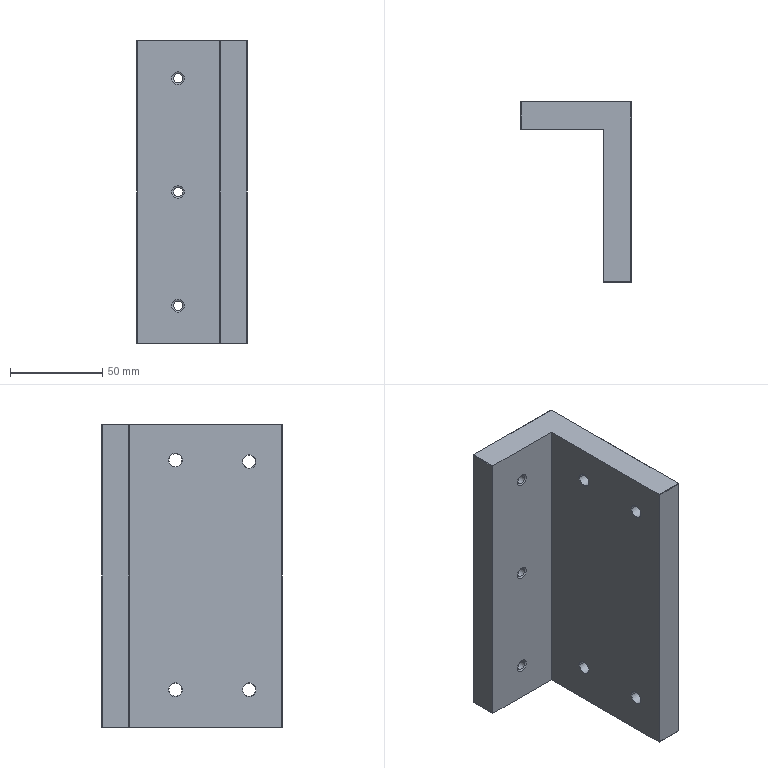Part | NX | 1 solid | 65 faces | box 60 x 98 x 164.5 mm | volume 349499 mm3 | cylinder 22 | cone 22 | plane 21 | commonest cylinder face diameters 2.5 x8 7 x8 5 x6